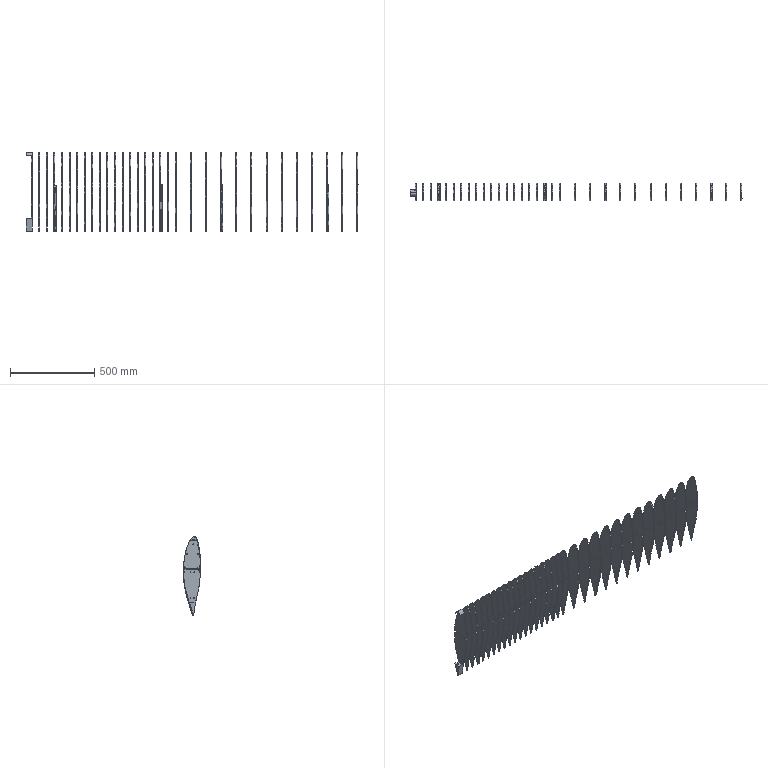Part | SolidWorks | features BaseBody 76 | 76 solids | 1477 faces | box 1972 x 103.205 x 466.085 mm | volume 6418827 mm3 | spline 1244 | plane 233